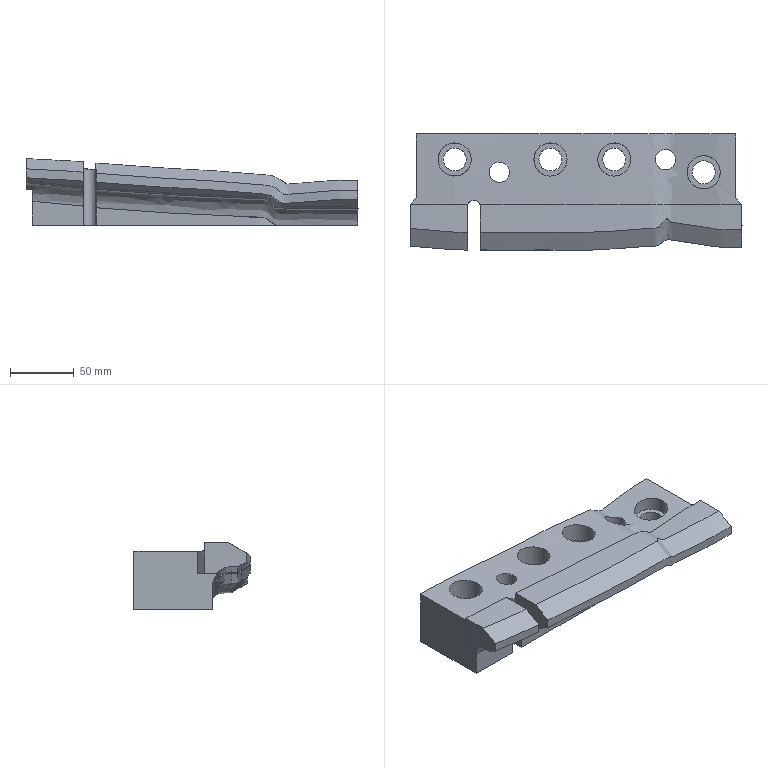Part | NX | features solid 2 | 1 solid | 59 faces | box 260 x 90.985 x 54.213 mm | volume 645996 mm3 | spline 31 | plane 17 | cylinder 11 | commonest cylinder face diameters 18 x4 26 x4 16 x2 10 x1